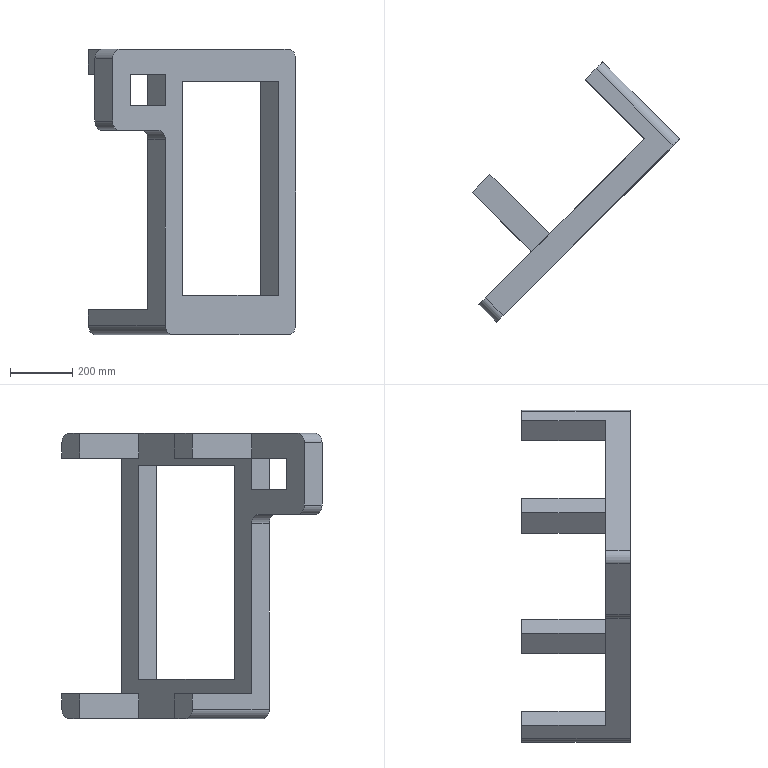Part | SolidWorks | 1 solid | 36 faces | box 666.188 x 835.894 x 917.42 mm | volume 30070373 mm3 | plane 30 | cylinder 6 | commonest cylinder face diameters 60 x6
STEP:
#1=CARTESIAN_POINT('',(-502.046,346.482,64.5));
#2=VERTEX_POINT('',#1);
#3=CARTESIAN_POINT('',(-502.046,346.482,-15.5));
#4=VERTEX_POINT('',#3);
#5=CARTESIAN_POINT('',(-502.046,346.482,64.5));
#6=DIRECTION('',(0.,0.,-1.));
#7=VECTOR('',#6,1000.);
#8=LINE('',#5,#7);
#9=EDGE_CURVE('',#2,#4,#8,.T.);
#10=ORIENTED_EDGE('',*,*,#9,.T.);
#11=CARTESIAN_POINT('',(-558.614,289.914,-15.5));
#12=VERTEX_POINT('',#11);
#13=CARTESIAN_POINT('',(-502.046,346.482,-15.5));
#14=DIRECTION('',(-0.7071,-0.7071,0.));
#15=VECTOR('',#14,1000.);
#16=LINE('',#13,#15);
#17=EDGE_CURVE('',#4,#12,#16,.T.);
#18=ORIENTED_EDGE('',*,*,#17,.T.);
#19=CARTESIAN_POINT('',(-558.614,289.914,64.5));
#20=VERTEX_POINT('',#19);
#21=CARTESIAN_POINT('',(-558.614,289.914,-15.5));
#22=DIRECTION('',(0.,0.,1.));
#23=VECTOR('',#22,1000.);
#24=LINE('',#21,#23);
#25=EDGE_CURVE('',#12,#20,#24,.T.);
#26=ORIENTED_EDGE('',*,*,#25,.T.);
#27=CARTESIAN_POINT('',(-558.614,289.914,64.5));
#28=DIRECTION('',(0.7071,0.7071,0.));
#29=VECTOR('',#28,1000.);
#30=LINE('',#27,#29);
#31=EDGE_CURVE('',#20,#2,#30,.T.);
#32=ORIENTED_EDGE('',*,*,#31,.T.);
#33=EDGE_LOOP('',(#10,#18,#26,#32));
#34=FACE_OUTER_BOUND('',#33,.T.);
#35=CARTESIAN_POINT('',(-424.264,424.264,0.));
#36=DIRECTION('',(-0.7071,0.7071,0.));
#37=DIRECTION('',(-0.7071,-0.7071,0.));
#38=AXIS2_PLACEMENT_3D('',#35,#36,#37);
#39=PLANE('',#38);
#40=ADVANCED_FACE('',(#34),#39,.T.);
#41=CARTESIAN_POINT('',(-311.127,155.563,64.5));
#42=VERTEX_POINT('',#41);
#43=CARTESIAN_POINT('',(-311.127,155.563,64.5));
#44=DIRECTION('',(-0.7071,0.7071,0.));
#45=VECTOR('',#44,1000.);
#46=LINE('',#43,#45);
#47=EDGE_CURVE('',#42,#2,#46,.T.);
#48=ORIENTED_EDGE('',*,*,#47,.T.);
#49=ORIENTED_EDGE('',*,*,#31,.F.);
#50=CARTESIAN_POINT('',(-367.696,98.995,64.5));
#51=VERTEX_POINT('',#50);
#52=CARTESIAN_POINT('',(-367.696,98.995,64.5));
#53=DIRECTION('',(-0.7071,0.7071,0.));
#54=VECTOR('',#53,1000.);
#55=LINE('',#52,#54);
#56=EDGE_CURVE('',#51,#20,#55,.T.);
#57=ORIENTED_EDGE('',*,*,#56,.F.);
#58=CARTESIAN_POINT('',(-367.696,98.995,64.5));
#59=DIRECTION('',(0.7071,0.7071,0.));
#60=VECTOR('',#59,1000.);
#61=LINE('',#58,#60);
#62=EDGE_CURVE('',#51,#42,#61,.T.);
#63=ORIENTED_EDGE('',*,*,#62,.T.);
#64=EDGE_LOOP('',(#48,#49,#57,#63));
#65=FACE_OUTER_BOUND('',#64,.T.);
#66=CARTESIAN_POINT('',(-311.127,42.426,64.5));
#67=DIRECTION('',(0.,0.,1.));
#68=DIRECTION('',(0.7071,0.7071,0.));
#69=AXIS2_PLACEMENT_3D('',#66,#67,#68);
#70=PLANE('',#69);
#71=ADVANCED_FACE('',(#65),#70,.T.);
#72=CARTESIAN_POINT('',(-311.127,155.563,-15.5));
#73=VERTEX_POINT('',#72);
#74=CARTESIAN_POINT('',(-311.127,155.563,-15.5));
#75=DIRECTION('',(-0.7071,0.7071,0.));
#76=VECTOR('',#75,1000.);
#77=LINE('',#74,#76);
#78=EDGE_CURVE('',#73,#4,#77,.T.);
#79=ORIENTED_EDGE('',*,*,#78,.T.);
#80=ORIENTED_EDGE('',*,*,#9,.F.);
#81=ORIENTED_EDGE('',*,*,#47,.F.);
#82=CARTESIAN_POINT('',(-311.127,155.563,64.5));
#83=DIRECTION('',(0.,0.,-1.));
#84=VECTOR('',#83,1000.);
#85=LINE('',#82,#84);
#86=EDGE_CURVE('',#42,#73,#85,.T.);
#87=ORIENTED_EDGE('',*,*,#86,.T.);
#88=EDGE_LOOP('',(#79,#80,#81,#87));
#89=FACE_OUTER_BOUND('',#88,.T.);
#90=CARTESIAN_POINT('',(-254.558,98.995,64.5));
#91=DIRECTION('',(0.7071,0.7071,0.));
#92=DIRECTION('',(0.,0.,-1.));
#93=AXIS2_PLACEMENT_3D('',#90,#91,#92);
#94=PLANE('',#93);
#95=ADVANCED_FACE('',(#89),#94,.T.);
#96=ORIENTED_EDGE('',*,*,#17,.F.);
#97=ORIENTED_EDGE('',*,*,#78,.F.);
#98=CARTESIAN_POINT('',(-367.696,98.995,-15.5));
#99=VERTEX_POINT('',#98);
#100=CARTESIAN_POINT('',(-311.127,155.563,-15.5));
#101=DIRECTION('',(-0.7071,-0.7071,0.));
#102=VECTOR('',#101,1000.);
#103=LINE('',#100,#102);
#104=EDGE_CURVE('',#73,#99,#103,.T.);
#105=ORIENTED_EDGE('',*,*,#104,.T.);
#106=CARTESIAN_POINT('',(-367.696,98.995,-15.5));
#107=DIRECTION('',(-0.7071,0.7071,0.));
#108=VECTOR('',#107,1000.);
#109=LINE('',#106,#108);
#110=EDGE_CURVE('',#99,#12,#109,.T.);
#111=ORIENTED_EDGE('',*,*,#110,.T.);
#112=EDGE_LOOP('',(#96,#97,#105,#111));
#113=FACE_OUTER_BOUND('',#112,.T.);
#114=CARTESIAN_POINT('',(-254.558,98.995,-15.5));
#115=DIRECTION('',(0.,0.,-1.));
#116=DIRECTION('',(-0.7071,-0.7071,0.));
#117=AXIS2_PLACEMENT_3D('',#114,#115,#116);
#118=PLANE('',#117);
#119=ADVANCED_FACE('',(#113),#118,.T.);
#120=ORIENTED_EDGE('',*,*,#56,.T.);
#121=ORIENTED_EDGE('',*,*,#25,.F.);
#122=ORIENTED_EDGE('',*,*,#110,.F.);
#123=CARTESIAN_POINT('',(-367.696,98.995,64.5));
#124=DIRECTION('',(0.,0.,-1.));
#125=VECTOR('',#124,1000.);
#126=LINE('',#123,#125);
#127=EDGE_CURVE('',#51,#99,#126,.T.);
#128=ORIENTED_EDGE('',*,*,#127,.F.);
#129=EDGE_LOOP('',(#120,#121,#122,#128));
#130=FACE_OUTER_BOUND('',#129,.T.);
#131=CARTESIAN_POINT('',(-311.127,42.426,-15.5));
#132=DIRECTION('',(-0.7071,-0.7071,0.));
#133=DIRECTION('',(0.,0.,1.));
#134=AXIS2_PLACEMENT_3D('',#131,#132,#133);
#135=PLANE('',#134);
#136=ADVANCED_FACE('',(#130),#135,.T.);
#137=CARTESIAN_POINT('',(-367.696,98.995,-115.5));
#138=VERTEX_POINT('',#137);
#139=CARTESIAN_POINT('',(-367.696,98.995,-15.5));
#140=DIRECTION('',(0.,0.,-1.));
#141=VECTOR('',#140,1000.);
#142=LINE('',#139,#141);
#143=EDGE_CURVE('',#99,#138,#142,.T.);
#144=ORIENTED_EDGE('',*,*,#143,.T.);
#145=CARTESIAN_POINT('',(-311.127,42.426,-115.5));
#146=VERTEX_POINT('',#145);
#147=CARTESIAN_POINT('',(-311.127,42.426,-115.5));
#148=DIRECTION('',(-0.7071,0.7071,0.));
#149=VECTOR('',#148,1000.);
#150=LINE('',#147,#149);
#151=EDGE_CURVE('',#146,#138,#150,.T.);
#152=ORIENTED_EDGE('',*,*,#151,.F.);
#153=CARTESIAN_POINT('',(-311.127,42.426,-15.5));
#154=VERTEX_POINT('',#153);
#155=CARTESIAN_POINT('',(-311.127,42.426,-15.5));
#156=DIRECTION('',(0.,0.,-1.));
#157=VECTOR('',#156,1000.);
#158=LINE('',#155,#157);
#159=EDGE_CURVE('',#154,#146,#158,.T.);
#160=ORIENTED_EDGE('',*,*,#159,.F.);
#161=CARTESIAN_POINT('',(-311.127,42.426,-15.5));
#162=DIRECTION('',(-0.7071,0.7071,0.));
#163=VECTOR('',#162,1000.);
#164=LINE('',#161,#163);
#165=EDGE_CURVE('',#154,#99,#164,.T.);
#166=ORIENTED_EDGE('',*,*,#165,.T.);
#167=EDGE_LOOP('',(#144,#152,#160,#166));
#168=FACE_OUTER_BOUND('',#167,.T.);
#169=CARTESIAN_POINT('',(-311.127,42.426,-15.5));
#170=DIRECTION('',(-0.7071,-0.7071,0.));
#171=DIRECTION('',(0.,0.,1.));
#172=AXIS2_PLACEMENT_3D('',#169,#170,#171);
#173=PLANE('',#172);
#174=ADVANCED_FACE('',(#168),#173,.T.);
#175=CARTESIAN_POINT('',(-424.264,-70.711,-115.5));
#176=VERTEX_POINT('',#175);
#177=CARTESIAN_POINT('',(-311.127,42.426,-115.5));
#178=DIRECTION('',(-0.7071,-0.7071,0.));
#179=VECTOR('',#178,1000.);
#180=LINE('',#177,#179);
#181=EDGE_CURVE('',#146,#176,#180,.T.);
#182=ORIENTED_EDGE('',*,*,#181,.F.);
#183=ORIENTED_EDGE('',*,*,#151,.T.);
#184=CARTESIAN_POINT('',(-480.833,-14.142,-115.5));
#185=VERTEX_POINT('',#184);
#186=CARTESIAN_POINT('',(-367.696,98.995,-115.5));
#187=DIRECTION('',(-0.7071,-0.7071,0.));
#188=VECTOR('',#187,1000.);
#189=LINE('',#186,#188);
#190=EDGE_CURVE('',#138,#185,#189,.T.);
#191=ORIENTED_EDGE('',*,*,#190,.T.);
#192=CARTESIAN_POINT('',(-424.264,-70.711,-115.5));
#193=DIRECTION('',(-0.7071,0.7071,0.));
#194=VECTOR('',#193,1000.);
#195=LINE('',#192,#194);
#196=EDGE_CURVE('',#176,#185,#195,.T.);
#197=ORIENTED_EDGE('',*,*,#196,.F.);
#198=EDGE_LOOP('',(#182,#183,#191,#197));
#199=FACE_OUTER_BOUND('',#198,.T.);
#200=CARTESIAN_POINT('',(-311.127,42.426,-115.5));
#201=DIRECTION('',(0.,0.,1.));
#202=DIRECTION('',(-0.7071,0.7071,0.));
#203=AXIS2_PLACEMENT_3D('',#200,#201,#202);
#204=PLANE('',#203);
#205=ADVANCED_FACE('',(#199),#204,.T.);
#206=CARTESIAN_POINT('',(-424.264,-70.711,-15.5));
#207=VERTEX_POINT('',#206);
#208=CARTESIAN_POINT('',(-424.264,-70.711,-15.5));
#209=DIRECTION('',(0.,0.,-1.));
#210=VECTOR('',#209,1000.);
#211=LINE('',#208,#210);
#212=EDGE_CURVE('',#207,#176,#211,.T.);
#213=ORIENTED_EDGE('',*,*,#212,.T.);
#214=ORIENTED_EDGE('',*,*,#196,.T.);
#215=CARTESIAN_POINT('',(-480.833,-14.142,-15.5));
#216=VERTEX_POINT('',#215);
#217=CARTESIAN_POINT('',(-480.833,-14.142,-15.5));
#218=DIRECTION('',(0.,0.,-1.));
#219=VECTOR('',#218,1000.);
#220=LINE('',#217,#219);
#221=EDGE_CURVE('',#216,#185,#220,.T.);
#222=ORIENTED_EDGE('',*,*,#221,.F.);
#223=CARTESIAN_POINT('',(-480.833,-14.142,-15.5));
#224=DIRECTION('',(0.7071,-0.7071,0.));
#225=VECTOR('',#224,1000.);
#226=LINE('',#223,#225);
#227=EDGE_CURVE('',#216,#207,#226,.T.);
#228=ORIENTED_EDGE('',*,*,#227,.T.);
#229=EDGE_LOOP('',(#213,#214,#222,#228));
#230=FACE_OUTER_BOUND('',#229,.T.);
#231=CARTESIAN_POINT('',(-424.264,-70.711,65.));
#232=DIRECTION('',(0.7071,0.7071,0.));
#233=DIRECTION('',(-0.7071,0.7071,0.));
#234=AXIS2_PLACEMENT_3D('',#231,#232,#233);
#235=PLANE('',#234);
#236=ADVANCED_FACE('',(#230),#235,.T.);
#237=CARTESIAN_POINT('',(-367.696,98.995,-15.5));
#238=DIRECTION('',(-0.7071,-0.7071,0.));
#239=VECTOR('',#238,1000.);
#240=LINE('',#237,#239);
#241=EDGE_CURVE('',#99,#216,#240,.T.);
#242=ORIENTED_EDGE('',*,*,#241,.F.);
#243=ORIENTED_EDGE('',*,*,#165,.F.);
#244=CARTESIAN_POINT('',(-311.127,42.426,-15.5));
#245=DIRECTION('',(-0.7071,-0.7071,0.));
#246=VECTOR('',#245,1000.);
#247=LINE('',#244,#246);
#248=EDGE_CURVE('',#154,#207,#247,.T.);
#249=ORIENTED_EDGE('',*,*,#248,.T.);
#250=ORIENTED_EDGE('',*,*,#227,.F.);
#251=EDGE_LOOP('',(#242,#243,#249,#250));
#252=FACE_OUTER_BOUND('',#251,.T.);
#253=CARTESIAN_POINT('',(-367.696,98.995,-15.5));
#254=DIRECTION('',(0.,0.,-1.));
#255=DIRECTION('',(0.7071,-0.7071,0.));
#256=AXIS2_PLACEMENT_3D('',#253,#254,#255);
#257=PLANE('',#256);
#258=ADVANCED_FACE('',(#252),#257,.T.);
#259=CARTESIAN_POINT('',(51.005,404.558,-726.128));
#260=VERTEX_POINT('',#259);
#261=CARTESIAN_POINT('',(-254.558,98.995,-726.128));
#262=VERTEX_POINT('',#261);
#263=CARTESIAN_POINT('',(51.005,404.558,-726.128));
#264=DIRECTION('',(-0.7071,-0.7071,0.));
#265=VECTOR('',#264,1000.);
#266=LINE('',#263,#265);
#267=EDGE_CURVE('',#260,#262,#266,.T.);
#268=ORIENTED_EDGE('',*,*,#267,.F.);
#269=CARTESIAN_POINT('',(-5.563,461.127,-726.128));
#270=VERTEX_POINT('',#269);
#271=CARTESIAN_POINT('',(51.005,404.558,-726.128));
#272=DIRECTION('',(-0.7071,0.7071,0.));
#273=VECTOR('',#272,1000.);
#274=LINE('',#271,#273);
#275=EDGE_CURVE('',#260,#270,#274,.T.);
#276=ORIENTED_EDGE('',*,*,#275,.T.);
#277=CARTESIAN_POINT('',(-311.127,155.563,-726.128));
#278=VERTEX_POINT('',#277);
#279=CARTESIAN_POINT('',(-5.563,461.127,-726.128));
#280=DIRECTION('',(-0.7071,-0.7071,0.));
#281=VECTOR('',#280,1000.);
#282=LINE('',#279,#281);
#283=EDGE_CURVE('',#270,#278,#282,.T.);
#284=ORIENTED_EDGE('',*,*,#283,.T.);
#285=CARTESIAN_POINT('',(-254.558,98.995,-726.128));
#286=DIRECTION('',(-0.7071,0.7071,0.));
#287=VECTOR('',#286,1000.);
#288=LINE('',#285,#287);
#289=EDGE_CURVE('',#262,#278,#288,.T.);
#290=ORIENTED_EDGE('',*,*,#289,.F.);
#291=EDGE_LOOP('',(#268,#276,#284,#290));
#292=FACE_OUTER_BOUND('',#291,.T.);
#293=CARTESIAN_POINT('',(51.005,517.696,-726.128));
#294=DIRECTION('',(0.,0.,1.));
#295=DIRECTION('',(0.7071,-0.7071,0.));
#296=AXIS2_PLACEMENT_3D('',#293,#294,#295);
#297=PLANE('',#296);
#298=ADVANCED_FACE('',(#292),#297,.T.);
#299=CARTESIAN_POINT('',(-5.563,461.127,-37.575));
#300=VERTEX_POINT('',#299);
#301=CARTESIAN_POINT('',(-5.563,461.127,-37.575));
#302=DIRECTION('',(0.,0.,-1.));
#303=VECTOR('',#302,1000.);
#304=LINE('',#301,#303);
#305=EDGE_CURVE('',#300,#270,#304,.T.);
#306=ORIENTED_EDGE('',*,*,#305,.T.);
#307=ORIENTED_EDGE('',*,*,#275,.F.);
#308=CARTESIAN_POINT('',(51.005,404.558,-37.575));
#309=VERTEX_POINT('',#308);
#310=CARTESIAN_POINT('',(51.005,404.558,-37.575));
#311=DIRECTION('',(0.,0.,-1.));
#312=VECTOR('',#311,1000.);
#313=LINE('',#310,#312);
#314=EDGE_CURVE('',#309,#260,#313,.T.);
#315=ORIENTED_EDGE('',*,*,#314,.F.);
#316=CARTESIAN_POINT('',(51.005,404.558,-37.575));
#317=DIRECTION('',(-0.7071,0.7071,0.));
#318=VECTOR('',#317,1000.);
#319=LINE('',#316,#318);
#320=EDGE_CURVE('',#309,#300,#319,.T.);
#321=ORIENTED_EDGE('',*,*,#320,.T.);
#322=EDGE_LOOP('',(#306,#307,#315,#321));
#323=FACE_OUTER_BOUND('',#322,.T.);
#324=CARTESIAN_POINT('',(51.005,404.558,-852.42));
#325=DIRECTION('',(-0.7071,-0.7071,0.));
#326=DIRECTION('',(0.,0.,1.));
#327=AXIS2_PLACEMENT_3D('',#324,#325,#326);
#328=PLANE('',#327);
#329=ADVANCED_FACE('',(#323),#328,.T.);
#330=CARTESIAN_POINT('',(-311.127,155.563,-37.575));
#331=VERTEX_POINT('',#330);
#332=CARTESIAN_POINT('',(-5.563,461.127,-37.575));
#333=DIRECTION('',(-0.7071,-0.7071,0.));
#334=VECTOR('',#333,1000.);
#335=LINE('',#332,#334);
#336=EDGE_CURVE('',#300,#331,#335,.T.);
#337=ORIENTED_EDGE('',*,*,#336,.F.);
#338=ORIENTED_EDGE('',*,*,#320,.F.);
#339=CARTESIAN_POINT('',(-254.558,98.995,-37.575));
#340=VERTEX_POINT('',#339);
#341=CARTESIAN_POINT('',(51.005,404.558,-37.575));
#342=DIRECTION('',(-0.7071,-0.7071,0.));
#343=VECTOR('',#342,1000.);
#344=LINE('',#341,#343);
#345=EDGE_CURVE('',#309,#340,#344,.T.);
#346=ORIENTED_EDGE('',*,*,#345,.T.);
#347=CARTESIAN_POINT('',(-254.558,98.995,-37.575));
#348=DIRECTION('',(-0.7071,0.7071,0.));
#349=VECTOR('',#348,1000.);
#350=LINE('',#347,#349);
#351=EDGE_CURVE('',#340,#331,#350,.T.);
#352=ORIENTED_EDGE('',*,*,#351,.T.);
#353=EDGE_LOOP('',(#337,#338,#346,#352));
#354=FACE_OUTER_BOUND('',#353,.T.);
#355=CARTESIAN_POINT('',(107.574,461.127,-37.575));
#356=DIRECTION('',(0.,0.,-1.));
#357=DIRECTION('',(-0.7071,0.7071,0.));
#358=AXIS2_PLACEMENT_3D('',#355,#356,#357);
#359=PLANE('',#358);
#360=ADVANCED_FACE('',(#354),#359,.T.);
#361=CARTESIAN_POINT('',(-254.558,98.995,-37.575));
#362=DIRECTION('',(0.,0.,-1.));
#363=VECTOR('',#362,1000.);
#364=LINE('',#361,#363);
#365=EDGE_CURVE('',#340,#262,#364,.T.);
#366=ORIENTED_EDGE('',*,*,#365,.T.);
#367=ORIENTED_EDGE('',*,*,#289,.T.);
#368=CARTESIAN_POINT('',(-311.127,155.563,-37.575));
#369=DIRECTION('',(0.,0.,-1.));
#370=VECTOR('',#369,1000.);
#371=LINE('',#368,#370);
#372=EDGE_CURVE('',#331,#278,#371,.T.);
#373=ORIENTED_EDGE('',*,*,#372,.F.);
#374=ORIENTED_EDGE('',*,*,#351,.F.);
#375=EDGE_LOOP('',(#366,#367,#373,#374));
#376=FACE_OUTER_BOUND('',#375,.T.);
#377=CARTESIAN_POINT('',(-254.558,98.995,64.5));
#378=DIRECTION('',(0.7071,0.7071,0.));
#379=DIRECTION('',(0.,0.,-1.));
#380=AXIS2_PLACEMENT_3D('',#377,#378,#379);
#381=PLANE('',#380);
#382=ADVANCED_FACE('',(#376),#381,.T.);
#383=CARTESIAN_POINT('',(-5.563,461.127,-15.));
#384=VERTEX_POINT('',#383);
#385=CARTESIAN_POINT('',(-196.482,652.046,-15.));
#386=VERTEX_POINT('',#385);
#387=CARTESIAN_POINT('',(-5.563,461.127,-15.));
#388=DIRECTION('',(-0.7071,0.7071,0.));
#389=VECTOR('',#388,1000.);
#390=LINE('',#387,#389);
#391=EDGE_CURVE('',#384,#386,#390,.T.);
#392=ORIENTED_EDGE('',*,*,#391,.T.);
#393=CARTESIAN_POINT('',(-139.914,708.614,-15.));
#394=VERTEX_POINT('',#393);
#395=CARTESIAN_POINT('',(-139.914,708.614,-15.));
#396=DIRECTION('',(-0.7071,-0.7071,0.));
#397=VECTOR('',#396,1000.);
#398=LINE('',#395,#397);
#399=EDGE_CURVE('',#394,#386,#398,.T.);
#400=ORIENTED_EDGE('',*,*,#399,.F.);
#401=CARTESIAN_POINT('',(51.005,517.696,-15.));
#402=VERTEX_POINT('',#401);
#403=CARTESIAN_POINT('',(51.005,517.696,-15.));
#404=DIRECTION('',(-0.7071,0.7071,0.));
#405=VECTOR('',#404,1000.);
#406=LINE('',#403,#405);
#407=EDGE_CURVE('',#402,#394,#406,.T.);
#408=ORIENTED_EDGE('',*,*,#407,.F.);
#409=CARTESIAN_POINT('',(51.005,517.696,-15.));
#410=DIRECTION('',(-0.7071,-0.7071,0.));
#411=VECTOR('',#410,1000.);
#412=LINE('',#409,#411);
#413=EDGE_CURVE('',#402,#384,#412,.T.);
#414=ORIENTED_EDGE('',*,*,#413,.T.);
#415=EDGE_LOOP('',(#392,#400,#408,#414));
#416=FACE_OUTER_BOUND('',#415,.T.);
#417=CARTESIAN_POINT('',(107.574,461.127,-15.));
#418=DIRECTION('',(0.,0.,-1.));
#419=DIRECTION('',(-0.7071,-0.7071,0.));
#420=AXIS2_PLACEMENT_3D('',#417,#418,#419);
#421=PLANE('',#420);
#422=ADVANCED_FACE('',(#416),#421,.T.);
#423=CARTESIAN_POINT('',(-502.046,346.482,-852.42));
#424=VERTEX_POINT('',#423);
#425=CARTESIAN_POINT('',(-537.401,311.127,-852.42));
#426=VERTEX_POINT('',#425);
#427=CARTESIAN_POINT('',(-502.046,346.482,-852.42));
#428=DIRECTION('',(-0.7071,-0.7071,0.));
#429=VECTOR('',#428,1000.);
#430=LINE('',#427,#429);
#431=EDGE_CURVE('',#424,#426,#430,.T.);
#432=ORIENTED_EDGE('',*,*,#431,.T.);
#433=CARTESIAN_POINT('',(-558.614,289.914,-822.42));
#434=VERTEX_POINT('',#433);
#435=CARTESIAN_POINT('',(-537.401,311.127,-822.42));
#436=DIRECTION('',(-0.7071,0.7071,0.));
#437=DIRECTION('',(-0.7071,-0.7071,0.));
#438=AXIS2_PLACEMENT_3D('',#435,#436,#437);
#439=CIRCLE('',#438,30.);
#440=EDGE_CURVE('',#426,#434,#439,.T.);
#441=ORIENTED_EDGE('',*,*,#440,.T.);
#442=CARTESIAN_POINT('',(-558.614,289.914,-772.42));
#443=VERTEX_POINT('',#442);
#444=CARTESIAN_POINT('',(-558.614,289.914,-852.42));
#445=DIRECTION('',(0.,0.,1.));
#446=VECTOR('',#445,1000.);
#447=LINE('',#444,#446);
#448=EDGE_CURVE('',#434,#443,#447,.T.);
#449=ORIENTED_EDGE('',*,*,#448,.T.);
#450=CARTESIAN_POINT('',(-502.046,346.482,-772.42));
#451=VERTEX_POINT('',#450);
#452=CARTESIAN_POINT('',(-558.614,289.914,-772.42));
#453=DIRECTION('',(0.7071,0.7071,0.));
#454=VECTOR('',#453,1000.);
#455=LINE('',#452,#454);
#456=EDGE_CURVE('',#443,#451,#455,.T.);
#457=ORIENTED_EDGE('',*,*,#456,.T.);
#458=CARTESIAN_POINT('',(-502.046,346.482,-772.42));
#459=DIRECTION('',(0.,0.,-1.));
#460=VECTOR('',#459,1000.);
#461=LINE('',#458,#460);
#462=EDGE_CURVE('',#451,#424,#461,.T.);
#463=ORIENTED_EDGE('',*,*,#462,.T.);
#464=EDGE_LOOP('',(#432,#441,#449,#457,#463));
#465=FACE_OUTER_BOUND('',#464,.T.);
#466=CARTESIAN_POINT('',(-424.264,424.264,0.));
#467=DIRECTION('',(-0.7071,0.7071,0.));
#468=DIRECTION('',(-0.7071,-0.7071,0.));
#469=AXIS2_PLACEMENT_3D('',#466,#467,#468);
#470=PLANE('',#469);
#471=ADVANCED_FACE('',(#465),#470,.T.);
#472=CARTESIAN_POINT('',(-332.34,21.213,-195.5));
#473=VERTEX_POINT('',#472);
#474=CARTESIAN_POINT('',(-459.619,-106.066,-195.5));
#475=VERTEX_POINT('',#474);
#476=CARTESIAN_POINT('',(-311.127,42.426,-195.5));
#477=DIRECTION('',(-0.7071,-0.7071,0.));
#478=VECTOR('',#477,1000.);
#479=LINE('',#476,#478);
#480=EDGE_CURVE('',#473,#475,#479,.T.);
#481=ORIENTED_EDGE('',*,*,#480,.T.);
#482=CARTESIAN_POINT('',(-516.188,-49.497,-195.5));
#483=VERTEX_POINT('',#482);
#484=CARTESIAN_POINT('',(-516.188,-49.497,-195.5));
#485=DIRECTION('',(-0.7071,0.7071,0.));
#486=VECTOR('',#485,1000.);
#487=LINE('',#484,#486);
#488=EDGE_CURVE('',#475,#483,#487,.T.);
#489=ORIENTED_EDGE('',*,*,#488,.T.);
#490=CARTESIAN_POINT('',(-388.909,77.782,-195.5));
#491=VERTEX_POINT('',#490);
#492=CARTESIAN_POINT('',(-367.696,98.995,-195.5));
#493=DIRECTION('',(-0.7071,-0.7071,0.));
#494=VECTOR('',#493,1000.);
#495=LINE('',#492,#494);
#496=EDGE_CURVE('',#491,#483,#495,.T.);
#497=ORIENTED_EDGE('',*,*,#496,.F.);
#498=CARTESIAN_POINT('',(-332.34,21.213,-195.5));
#499=DIRECTION('',(0.7071,-0.7071,0.));
#500=VECTOR('',#499,1000.);
#501=LINE('',#498,#500);
#502=EDGE_CURVE('',#491,#473,#501,.T.);
#503=ORIENTED_EDGE('',*,*,#502,.T.);
#504=EDGE_LOOP('',(#481,#489,#497,#503));
#505=FACE_OUTER_BOUND('',#504,.T.);
#506=CARTESIAN_POINT('',(-367.696,98.995,-195.5));
#507=DIRECTION('',(0.,0.,-1.));
#508=DIRECTION('',(0.7071,-0.7071,0.));
#509=AXIS2_PLACEMENT_3D('',#506,#507,#508);
#510=PLANE('',#509);
#511=ADVANCED_FACE('',(#505),#510,.T.);
#512=ORIENTED_EDGE('',*,*,#448,.F.);
#513=CARTESIAN_POINT('',(-311.127,42.426,-822.42));
#514=VERTEX_POINT('',#513);
#515=CARTESIAN_POINT('',(-311.127,42.426,-822.42));
#516=DIRECTION('',(0.7071,-0.7071,0.));
#517=VECTOR('',#516,1000.);
#518=LINE('',#515,#517);
#519=EDGE_CURVE('',#434,#514,#518,.T.);
#520=ORIENTED_EDGE('',*,*,#519,.T.);
#521=CARTESIAN_POINT('',(-311.127,42.426,-225.5));
#522=VERTEX_POINT('',#521);
#523=CARTESIAN_POINT('',(-311.127,42.426,-195.5));
#524=DIRECTION('',(0.,0.,-1.));
#525=VECTOR('',#524,1000.);
#526=LINE('',#523,#525);
#527=EDGE_CURVE('',#522,#514,#526,.T.);
#528=ORIENTED_EDGE('',*,*,#527,.F.);
#529=CARTESIAN_POINT('',(-367.696,98.995,-225.5));
#530=VERTEX_POINT('',#529);
#531=CARTESIAN_POINT('',(-367.696,98.995,-225.5));
#532=DIRECTION('',(-0.7071,0.7071,0.));
#533=VECTOR('',#532,1000.);
#534=LINE('',#531,#533);
#535=EDGE_CURVE('',#522,#530,#534,.T.);
#536=ORIENTED_EDGE('',*,*,#535,.T.);
#537=CARTESIAN_POINT('',(-367.696,98.995,-772.42));
#538=VERTEX_POINT('',#537);
#539=CARTESIAN_POINT('',(-367.696,98.995,-195.5));
#540=DIRECTION('',(0.,0.,-1.));
#541=VECTOR('',#540,1000.);
#542=LINE('',#539,#541);
#543=EDGE_CURVE('',#530,#538,#542,.T.);
#544=ORIENTED_EDGE('',*,*,#543,.T.);
#545=CARTESIAN_POINT('',(-367.696,98.995,-772.42));
#546=DIRECTION('',(-0.7071,0.7071,0.));
#547=VECTOR('',#546,1000.);
#548=LINE('',#545,#547);
#549=EDGE_CURVE('',#538,#443,#548,.T.);
#550=ORIENTED_EDGE('',*,*,#549,.T.);
#551=EDGE_LOOP('',(#512,#520,#528,#536,#544,#550));
#552=FACE_OUTER_BOUND('',#551,.T.);
#553=CARTESIAN_POINT('',(-311.127,42.426,-15.5));
#554=DIRECTION('',(-0.7071,-0.7071,0.));
#555=DIRECTION('',(0.,0.,1.));
#556=AXIS2_PLACEMENT_3D('',#553,#554,#555);
#557=PLANE('',#556);
#558=ADVANCED_FACE('',(#552),#557,.T.);
#559=CARTESIAN_POINT('',(-311.127,155.563,-772.42));
#560=VERTEX_POINT('',#559);
#561=CARTESIAN_POINT('',(-311.127,155.563,-772.42));
#562=DIRECTION('',(-0.7071,0.7071,0.));
#563=VECTOR('',#562,1000.);
#564=LINE('',#561,#563);
#565=EDGE_CURVE('',#560,#451,#564,.T.);
#566=ORIENTED_EDGE('',*,*,#565,.T.);
#567=ORIENTED_EDGE('',*,*,#456,.F.);
#568=ORIENTED_EDGE('',*,*,#549,.F.);
#569=CARTESIAN_POINT('',(-367.696,98.995,-772.42));
#570=DIRECTION('',(0.7071,0.7071,0.));
#571=VECTOR('',#570,1000.);
#572=LINE('',#569,#571);
#573=EDGE_CURVE('',#538,#560,#572,.T.);
#574=ORIENTED_EDGE('',*,*,#573,.T.);
#575=EDGE_LOOP('',(#566,#567,#568,#574));
#576=FACE_OUTER_BOUND('',#575,.T.);
#577=CARTESIAN_POINT('',(-311.127,42.426,-772.42));
#578=DIRECTION('',(0.,0.,1.));
#579=DIRECTION('',(0.7071,0.7071,0.));
#580=AXIS2_PLACEMENT_3D('',#577,#578,#579);
#581=PLANE('',#580);
#582=ADVANCED_FACE('',(#576),#581,.T.);
#583=CARTESIAN_POINT('',(-311.127,155.563,-852.42));
#584=VERTEX_POINT('',#583);
#585=CARTESIAN_POINT('',(-311.127,155.563,-852.42));
#586=DIRECTION('',(-0.7071,0.7071,0.));
#587=VECTOR('',#586,1000.);
#588=LINE('',#585,#587);
#589=EDGE_CURVE('',#584,#424,#588,.T.);
#590=ORIENTED_EDGE('',*,*,#589,.T.);
#591=ORIENTED_EDGE('',*,*,#462,.F.);
#592=ORIENTED_EDGE('',*,*,#565,.F.);
#593=CARTESIAN_POINT('',(-311.127,155.563,-852.42));
#594=DIRECTION('',(0.,0.,1.));
#595=VECTOR('',#594,1000.);
#596=LINE('',#593,#595);
#597=EDGE_CURVE('',#584,#560,#596,.T.);
#598=ORIENTED_EDGE('',*,*,#597,.F.);
#599=EDGE_LOOP('',(#590,#591,#592,#598));
#600=FACE_OUTER_BOUND('',#599,.T.);
#601=CARTESIAN_POINT('',(-254.558,98.995,64.5));
#602=DIRECTION('',(0.7071,0.7071,0.));
#603=DIRECTION('',(0.,0.,-1.));
#604=AXIS2_PLACEMENT_3D('',#601,#602,#603);
#605=PLANE('',#604);
#606=ADVANCED_FACE('',(#600),#605,.T.);
#607=CARTESIAN_POINT('',(-139.914,708.614,-772.42));
#608=VERTEX_POINT('',#607);
#609=CARTESIAN_POINT('',(-139.914,708.614,-822.42));
#610=VERTEX_POINT('',#609);
#611=CARTESIAN_POINT('',(-139.914,708.614,-772.42));
#612=DIRECTION('',(0.,0.,-1.));
#613=VECTOR('',#612,1000.);
#614=LINE('',#611,#613);
#615=EDGE_CURVE('',#608,#610,#614,.T.);
#616=ORIENTED_EDGE('',*,*,#615,.T.);
#617=CARTESIAN_POINT('',(-161.127,687.401,-852.42));
#618=VERTEX_POINT('',#617);
#619=CARTESIAN_POINT('',(-161.127,687.401,-822.42));
#620=DIRECTION('',(-0.7071,0.7071,0.));
#621=DIRECTION('',(-0.7071,-0.7071,0.));
#622=AXIS2_PLACEMENT_3D('',#619,#620,#621);
#623=CIRCLE('',#622,30.);
#624=EDGE_CURVE('',#610,#618,#623,.T.);
#625=ORIENTED_EDGE('',*,*,#624,.T.);
#626=CARTESIAN_POINT('',(-196.482,652.046,-852.42));
#627=VERTEX_POINT('',#626);
#628=CARTESIAN_POINT('',(-139.914,708.614,-852.42));
#629=DIRECTION('',(-0.7071,-0.7071,0.));
#630=VECTOR('',#629,1000.);
#631=LINE('',#628,#630);
#632=EDGE_CURVE('',#618,#627,#631,.T.);
#633=ORIENTED_EDGE('',*,*,#632,.T.);
#634=CARTESIAN_POINT('',(-196.482,652.046,-772.42));
#635=VERTEX_POINT('',#634);
#636=CARTESIAN_POINT('',(-196.482,652.046,-852.42));
#637=DIRECTION('',(0.,0.,1.));
#638=VECTOR('',#637,1000.);
#639=LINE('',#636,#638);
#640=EDGE_CURVE('',#627,#635,#639,.T.);
#641=ORIENTED_EDGE('',*,*,#640,.T.);
#642=CARTESIAN_POINT('',(-196.482,652.046,-772.42));
#643=DIRECTION('',(0.7071,0.7071,0.));
#644=VECTOR('',#643,1000.);
#645=LINE('',#642,#644);
#646=EDGE_CURVE('',#635,#608,#645,.T.);
#647=ORIENTED_EDGE('',*,*,#646,.T.);
#648=EDGE_LOOP('',(#616,#625,#633,#641,#647));
#649=FACE_OUTER_BOUND('',#648,.T.);
#650=CARTESIAN_POINT('',(-424.264,424.264,0.));
#651=DIRECTION('',(-0.7071,0.7071,0.));
#652=DIRECTION('',(-0.7071,-0.7071,0.));
#653=AXIS2_PLACEMENT_3D('',#650,#651,#652);
#654=PLANE('',#653);
#655=ADVANCED_FACE('',(#649),#654,.T.);
#656=CARTESIAN_POINT('',(-289.914,63.64,-852.42));
#657=VERTEX_POINT('',#656);
#658=CARTESIAN_POINT('',(86.36,439.914,-852.42));
#659=VERTEX_POINT('',#658);
#660=CARTESIAN_POINT('',(-311.127,42.426,-852.42));
#661=DIRECTION('',(0.7071,0.7071,0.));
#662=VECTOR('',#661,1000.);
#663=LINE('',#660,#662);
#664=EDGE_CURVE('',#657,#659,#663,.T.);
#665=ORIENTED_EDGE('',*,*,#664,.F.);
#666=CARTESIAN_POINT('',(-289.914,63.64,-852.42));
#667=DIRECTION('',(-0.7071,0.7071,0.));
#668=VECTOR('',#667,1000.);
#669=LINE('',#666,#668);
#670=EDGE_CURVE('',#657,#426,#669,.T.);
#671=ORIENTED_EDGE('',*,*,#670,.T.);
#672=ORIENTED_EDGE('',*,*,#431,.F.);
#673=ORIENTED_EDGE('',*,*,#589,.F.);
#674=CARTESIAN_POINT('',(-5.563,461.127,-852.42));
#675=VERTEX_POINT('',#674);
#676=CARTESIAN_POINT('',(-5.563,461.127,-852.42));
#677=DIRECTION('',(-0.7071,-0.7071,0.));
#678=VECTOR('',#677,1000.);
#679=LINE('',#676,#678);
#680=EDGE_CURVE('',#675,#584,#679,.T.);
#681=ORIENTED_EDGE('',*,*,#680,.F.);
#682=CARTESIAN_POINT('',(-5.563,461.127,-852.42));
#683=DIRECTION('',(-0.7071,0.7071,0.));
#684=VECTOR('',#683,1000.);
#685=LINE('',#682,#684);
#686=EDGE_CURVE('',#675,#627,#685,.T.);
#687=ORIENTED_EDGE('',*,*,#686,.T.);
#688=ORIENTED_EDGE('',*,*,#632,.F.);
#689=CARTESIAN_POINT('',(86.36,439.914,-852.42));
#690=DIRECTION('',(0.7071,-0.7071,0.));
#691=VECTOR('',#690,1000.);
#692=LINE('',#689,#691);
#693=EDGE_CURVE('',#618,#659,#692,.T.);
#694=ORIENTED_EDGE('',*,*,#693,.T.);
#695=EDGE_LOOP('',(#665,#671,#672,#673,#681,#687,#688,#694));
#696=FACE_OUTER_BOUND('',#695,.T.);
#697=CARTESIAN_POINT('',(-254.558,98.995,-852.42));
#698=DIRECTION('',(0.,0.,-1.));
#699=DIRECTION('',(-0.7071,-0.7071,0.));
#700=AXIS2_PLACEMENT_3D('',#697,#698,#699);
#701=PLANE('',#700);
#702=ADVANCED_FACE('',(#696),#701,.T.);
#703=CARTESIAN_POINT('',(-5.563,461.127,-772.42));
#704=VERTEX_POINT('',#703);
#705=CARTESIAN_POINT('',(-5.563,461.127,-772.42));
#706=DIRECTION('',(-0.7071,0.7071,0.));
#707=VECTOR('',#706,1000.);
#708=LINE('',#705,#707);
#709=EDGE_CURVE('',#704,#635,#708,.T.);
#710=ORIENTED_EDGE('',*,*,#709,.T.);
#711=ORIENTED_EDGE('',*,*,#640,.F.);
#712=ORIENTED_EDGE('',*,*,#686,.F.);
#713=CARTESIAN_POINT('',(-5.563,461.127,-852.42));
#714=DIRECTION('',(0.,0.,1.));
#715=VECTOR('',#714,1000.);
#716=LINE('',#713,#715);
#717=EDGE_CURVE('',#675,#704,#716,.T.);
#718=ORIENTED_EDGE('',*,*,#717,.T.);
#719=EDGE_LOOP('',(#710,#711,#712,#718));
#720=FACE_OUTER_BOUND('',#719,.T.);
#721=CARTESIAN_POINT('',(51.005,404.558,-852.42));
#722=DIRECTION('',(-0.7071,-0.7071,0.));
#723=DIRECTION('',(0.,0.,1.));
#724=AXIS2_PLACEMENT_3D('',#721,#722,#723);
#725=PLANE('',#724);
#726=ADVANCED_FACE('',(#720),#725,.T.);
#727=CARTESIAN_POINT('',(51.005,517.696,-772.42));
#728=VERTEX_POINT('',#727);
#729=CARTESIAN_POINT('',(51.005,517.696,-772.42));
#730=DIRECTION('',(-0.7071,0.7071,0.));
#731=VECTOR('',#730,1000.);
#732=LINE('',#729,#731);
#733=EDGE_CURVE('',#728,#608,#732,.T.);
#734=ORIENTED_EDGE('',*,*,#733,.T.);
#735=ORIENTED_EDGE('',*,*,#646,.F.);
#736=ORIENTED_EDGE('',*,*,#709,.F.);
#737=CARTESIAN_POINT('',(-5.563,461.127,-772.42));
#738=DIRECTION('',(0.7071,0.7071,0.));
#739=VECTOR('',#738,1000.);
#740=LINE('',#737,#739);
#741=EDGE_CURVE('',#704,#728,#740,.T.);
#742=ORIENTED_EDGE('',*,*,#741,.T.);
#743=EDGE_LOOP('',(#734,#735,#736,#742));
#744=FACE_OUTER_BOUND('',#743,.T.);
#745=CARTESIAN_POINT('',(51.005,404.558,-772.42));
#746=DIRECTION('',(0.,0.,1.));
#747=DIRECTION('',(0.7071,0.7071,0.));
#748=AXIS2_PLACEMENT_3D('',#745,#746,#747);
#749=PLANE('',#748);
#750=ADVANCED_FACE('',(#744),#749,.T.);
#751=CARTESIAN_POINT('',(-139.914,708.614,35.));
#752=VERTEX_POINT('',#751);
#753=CARTESIAN_POINT('',(-139.914,708.614,65.));
#754=DIRECTION('',(0.,0.,-1.));
#755=VECTOR('',#754,1000.);
#756=LINE('',#753,#755);
#757=EDGE_CURVE('',#752,#394,#756,.T.);
#758=ORIENTED_EDGE('',*,*,#757,.F.);
#759=CARTESIAN_POINT('',(107.574,461.127,35.));
#760=VERTEX_POINT('',#759);
#761=CARTESIAN_POINT('',(107.574,461.127,35.));
#762=DIRECTION('',(0.7071,-0.7071,0.));
#763=VECTOR('',#762,1000.);
#764=LINE('',#761,#763);
#765=EDGE_CURVE('',#752,#760,#764,.T.);
#766=ORIENTED_EDGE('',*,*,#765,.T.);
#767=CARTESIAN_POINT('',(107.574,461.127,-822.42));
#768=VERTEX_POINT('',#767);
#769=CARTESIAN_POINT('',(107.574,461.127,65.));
#770=DIRECTION('',(0.,0.,-1.));
#771=VECTOR('',#770,1000.);
#772=LINE('',#769,#771);
#773=EDGE_CURVE('',#760,#768,#772,.T.);
#774=ORIENTED_EDGE('',*,*,#773,.T.);
#775=CARTESIAN_POINT('',(107.574,461.127,-822.42));
#776=DIRECTION('',(-0.7071,0.7071,0.));
#777=VECTOR('',#776,1000.);
#778=LINE('',#775,#777);
#779=EDGE_CURVE('',#768,#610,#778,.T.);
#780=ORIENTED_EDGE('',*,*,#779,.T.);
#781=ORIENTED_EDGE('',*,*,#615,.F.);
#782=ORIENTED_EDGE('',*,*,#733,.F.);
#783=CARTESIAN_POINT('',(51.005,517.696,-772.42));
#784=DIRECTION('',(0.,0.,1.));
#785=VECTOR('',#784,1000.);
#786=LINE('',#783,#785);
#787=EDGE_CURVE('',#728,#402,#786,.T.);
#788=ORIENTED_EDGE('',*,*,#787,.T.);
#789=ORIENTED_EDGE('',*,*,#407,.T.);
#790=EDGE_LOOP('',(#758,#766,#774,#780,#781,#782,#788,#789));
#791=FACE_OUTER_BOUND('',#790,.T.);
#792=CARTESIAN_POINT('',(107.574,461.127,65.));
#793=DIRECTION('',(0.7071,0.7071,0.));
#794=DIRECTION('',(0.,0.,-1.));
#795=AXIS2_PLACEMENT_3D('',#792,#793,#794);
#796=PLANE('',#795);
#797=ADVANCED_FACE('',(#791),#796,.T.);
#798=CARTESIAN_POINT('',(-196.482,652.046,65.));
#799=VERTEX_POINT('',#798);
#800=CARTESIAN_POINT('',(-161.127,687.401,65.));
#801=VERTEX_POINT('',#800);
#802=CARTESIAN_POINT('',(-196.482,652.046,65.));
#803=DIRECTION('',(0.7071,0.7071,0.));
#804=VECTOR('',#803,1000.);
#805=LINE('',#802,#804);
#806=EDGE_CURVE('',#799,#801,#805,.T.);
#807=ORIENTED_EDGE('',*,*,#806,.T.);
#808=CARTESIAN_POINT('',(-161.127,687.401,35.));
#809=DIRECTION('',(-0.7071,0.7071,0.));
#810=DIRECTION('',(-0.7071,-0.7071,0.));
#811=AXIS2_PLACEMENT_3D('',#808,#809,#810);
#812=CIRCLE('',#811,30.);
#813=EDGE_CURVE('',#801,#752,#812,.T.);
#814=ORIENTED_EDGE('',*,*,#813,.T.);
#815=ORIENTED_EDGE('',*,*,#757,.T.);
#816=ORIENTED_EDGE('',*,*,#399,.T.);
#817=CARTESIAN_POINT('',(-196.482,652.046,-15.));
#818=DIRECTION('',(0.,0.,1.));
#819=VECTOR('',#818,1000.);
#820=LINE('',#817,#819);
#821=EDGE_CURVE('',#386,#799,#820,.T.);
#822=ORIENTED_EDGE('',*,*,#821,.T.);
#823=EDGE_LOOP('',(#807,#814,#815,#816,#822));
#824=FACE_OUTER_BOUND('',#823,.T.);
#825=CARTESIAN_POINT('',(-424.264,424.264,0.));
#826=DIRECTION('',(-0.7071,0.7071,0.));
#827=DIRECTION('',(-0.7071,-0.7071,0.));
#828=AXIS2_PLACEMENT_3D('',#825,#826,#827);
#829=PLANE('',#828);
#830=ADVANCED_FACE('',(#824),#829,.T.);
#831=CARTESIAN_POINT('',(-5.563,461.127,65.));
#832=VERTEX_POINT('',#831);
#833=CARTESIAN_POINT('',(-516.188,-49.497,65.));
#834=VERTEX_POINT('',#833);
#835=CARTESIAN_POINT('',(-5.563,461.127,65.));
#836=DIRECTION('',(-0.7071,-0.7071,0.));
#837=VECTOR('',#836,1000.);
#838=LINE('',#835,#837);
#839=EDGE_CURVE('',#832,#834,#838,.T.);
#840=ORIENTED_EDGE('',*,*,#839,.T.);
#841=CARTESIAN_POINT('',(-459.619,-106.066,65.));
#842=VERTEX_POINT('',#841);
#843=CARTESIAN_POINT('',(-459.619,-106.066,65.));
#844=DIRECTION('',(0.7071,-0.7071,0.));
#845=VECTOR('',#844,1000.);
#846=LINE('',#843,#845);
#847=EDGE_CURVE('',#834,#842,#846,.T.);
#848=ORIENTED_EDGE('',*,*,#847,.T.);
#849=CARTESIAN_POINT('',(86.36,439.914,65.));
#850=VERTEX_POINT('',#849);
#851=CARTESIAN_POINT('',(-480.833,-127.279,65.));
#852=DIRECTION('',(0.7071,0.7071,0.));
#853=VECTOR('',#852,1000.);
#854=LINE('',#851,#853);
#855=EDGE_CURVE('',#842,#850,#854,.T.);
#856=ORIENTED_EDGE('',*,*,#855,.T.);
#857=CARTESIAN_POINT('',(86.36,439.914,65.));
#858=DIRECTION('',(-0.7071,0.7071,0.));
#859=VECTOR('',#858,1000.);
#860=LINE('',#857,#859);
#861=EDGE_CURVE('',#850,#801,#860,.T.);
#862=ORIENTED_EDGE('',*,*,#861,.T.);
#863=ORIENTED_EDGE('',*,*,#806,.F.);
#864=CARTESIAN_POINT('',(-5.563,461.127,65.));
#865=DIRECTION('',(-0.7071,0.7071,0.));
#866=VECTOR('',#865,1000.);
#867=LINE('',#864,#866);
#868=EDGE_CURVE('',#832,#799,#867,.T.);
#869=ORIENTED_EDGE('',*,*,#868,.F.);
#870=EDGE_LOOP('',(#840,#848,#856,#862,#863,#869));
#871=FACE_OUTER_BOUND('',#870,.T.);
#872=CARTESIAN_POINT('',(51.005,404.558,65.));
#873=DIRECTION('',(0.,0.,1.));
#874=DIRECTION('',(0.7071,0.7071,0.));
#875=AXIS2_PLACEMENT_3D('',#872,#873,#874);
#876=PLANE('',#875);
#877=ADVANCED_FACE('',(#871),#876,.T.);
#878=ORIENTED_EDGE('',*,*,#159,.T.);
#879=ORIENTED_EDGE('',*,*,#181,.T.);
#880=ORIENTED_EDGE('',*,*,#212,.F.);
#881=ORIENTED_EDGE('',*,*,#248,.F.);
#882=EDGE_LOOP('',(#878,#879,#880,#881));
#883=FACE_BOUND('',#882,.T.);
#884=ORIENTED_EDGE('',*,*,#345,.F.);
#885=ORIENTED_EDGE('',*,*,#314,.T.);
#886=ORIENTED_EDGE('',*,*,#267,.T.);
#887=ORIENTED_EDGE('',*,*,#365,.F.);
#888=EDGE_LOOP('',(#884,#885,#886,#887));
#889=FACE_BOUND('',#888,.T.);
#890=CARTESIAN_POINT('',(-480.833,-127.279,-165.5));
#891=VERTEX_POINT('',#890);
#892=CARTESIAN_POINT('',(-480.833,-127.279,35.));
#893=VERTEX_POINT('',#892);
#894=CARTESIAN_POINT('',(-480.833,-127.279,-195.5));
#895=DIRECTION('',(0.,0.,1.));
#896=VECTOR('',#895,1000.);
#897=LINE('',#894,#896);
#898=EDGE_CURVE('',#891,#893,#897,.T.);
#899=ORIENTED_EDGE('',*,*,#898,.F.);
#900=CARTESIAN_POINT('',(-459.619,-106.066,-165.5));
#901=DIRECTION('',(0.7071,-0.7071,0.));
#902=DIRECTION('',(-0.7071,-0.7071,0.));
#903=AXIS2_PLACEMENT_3D('',#900,#901,#902);
#904=CIRCLE('',#903,30.);
#905=EDGE_CURVE('',#891,#475,#904,.T.);
#906=ORIENTED_EDGE('',*,*,#905,.T.);
#907=ORIENTED_EDGE('',*,*,#480,.F.);
#908=CARTESIAN_POINT('',(-332.34,21.213,-225.5));
#909=DIRECTION('',(-0.7071,0.7071,0.));
#910=DIRECTION('',(-0.7071,-0.7071,0.));
#911=AXIS2_PLACEMENT_3D('',#908,#909,#910);
#912=CIRCLE('',#911,30.);
#913=EDGE_CURVE('',#473,#522,#912,.T.);
#914=ORIENTED_EDGE('',*,*,#913,.T.);
#915=ORIENTED_EDGE('',*,*,#527,.T.);
#916=CARTESIAN_POINT('',(-289.914,63.64,-822.42));
#917=DIRECTION('',(0.7071,-0.7071,0.));
#918=DIRECTION('',(-0.7071,-0.7071,0.));
#919=AXIS2_PLACEMENT_3D('',#916,#917,#918);
#920=CIRCLE('',#919,30.);
#921=EDGE_CURVE('',#514,#657,#920,.T.);
#922=ORIENTED_EDGE('',*,*,#921,.T.);
#923=ORIENTED_EDGE('',*,*,#664,.T.);
#924=CARTESIAN_POINT('',(86.36,439.914,-822.42));
#925=DIRECTION('',(0.7071,-0.7071,0.));
#926=DIRECTION('',(-0.7071,-0.7071,0.));
#927=AXIS2_PLACEMENT_3D('',#924,#925,#926);
#928=CIRCLE('',#927,30.);
#929=EDGE_CURVE('',#659,#768,#928,.T.);
#930=ORIENTED_EDGE('',*,*,#929,.T.);
#931=ORIENTED_EDGE('',*,*,#773,.F.);
#932=CARTESIAN_POINT('',(86.36,439.914,35.));
#933=DIRECTION('',(0.7071,-0.7071,0.));
#934=DIRECTION('',(-0.7071,-0.7071,0.));
#935=AXIS2_PLACEMENT_3D('',#932,#933,#934);
#936=CIRCLE('',#935,30.);
#937=EDGE_CURVE('',#760,#850,#936,.T.);
#938=ORIENTED_EDGE('',*,*,#937,.T.);
#939=ORIENTED_EDGE('',*,*,#855,.F.);
#940=CARTESIAN_POINT('',(-459.619,-106.066,35.));
#941=DIRECTION('',(0.7071,-0.7071,0.));
#942=DIRECTION('',(-0.7071,-0.7071,0.));
#943=AXIS2_PLACEMENT_3D('',#940,#941,#942);
#944=CIRCLE('',#943,30.);
#945=EDGE_CURVE('',#842,#893,#944,.T.);
#946=ORIENTED_EDGE('',*,*,#945,.T.);
#947=EDGE_LOOP('',(#899,#906,#907,#914,#915,#922,#923,#930,#931,#938,#939,#946));
#948=FACE_OUTER_BOUND('',#947,.T.);
#949=CARTESIAN_POINT('',(-176.777,176.777,0.));
#950=DIRECTION('',(-0.7071,0.7071,0.));
#951=DIRECTION('',(-0.7071,-0.7071,0.));
#952=AXIS2_PLACEMENT_3D('',#949,#950,#951);
#953=PLANE('',#952);
#954=ADVANCED_FACE('',(#883,#889,#948),#953,.F.);
#955=CARTESIAN_POINT('',(-537.401,-70.711,35.));
#956=VERTEX_POINT('',#955);
#957=CARTESIAN_POINT('',(-537.401,-70.711,-165.5));
#958=VERTEX_POINT('',#957);
#959=CARTESIAN_POINT('',(-537.401,-70.711,65.));
#960=DIRECTION('',(0.,0.,-1.));
#961=VECTOR('',#960,1000.);
#962=LINE('',#959,#961);
#963=EDGE_CURVE('',#956,#958,#962,.T.);
#964=ORIENTED_EDGE('',*,*,#963,.T.);
#965=CARTESIAN_POINT('',(-480.833,-127.279,-165.5));
#966=DIRECTION('',(0.7071,-0.7071,0.));
#967=VECTOR('',#966,1000.);
#968=LINE('',#965,#967);
#969=EDGE_CURVE('',#958,#891,#968,.T.);
#970=ORIENTED_EDGE('',*,*,#969,.T.);
#971=ORIENTED_EDGE('',*,*,#898,.T.);
#972=CARTESIAN_POINT('',(-537.401,-70.711,35.));
#973=DIRECTION('',(-0.7071,0.7071,0.));
#974=VECTOR('',#973,1000.);
#975=LINE('',#972,#974);
#976=EDGE_CURVE('',#893,#956,#975,.T.);
#977=ORIENTED_EDGE('',*,*,#976,.T.);
#978=EDGE_LOOP('',(#964,#970,#971,#977));
#979=FACE_OUTER_BOUND('',#978,.T.);
#980=CARTESIAN_POINT('',(-466.69,-141.421,64.5));
#981=DIRECTION('',(0.7071,0.7071,0.));
#982=DIRECTION('',(0.,0.,1.));
#983=AXIS2_PLACEMENT_3D('',#980,#981,#982);
#984=PLANE('',#983);
#985=ADVANCED_FACE('',(#979),#984,.F.);
#986=ORIENTED_EDGE('',*,*,#143,.F.);
#987=ORIENTED_EDGE('',*,*,#104,.F.);
#988=ORIENTED_EDGE('',*,*,#86,.F.);
#989=ORIENTED_EDGE('',*,*,#62,.F.);
#990=ORIENTED_EDGE('',*,*,#127,.T.);
#991=ORIENTED_EDGE('',*,*,#241,.T.);
#992=ORIENTED_EDGE('',*,*,#221,.T.);
#993=ORIENTED_EDGE('',*,*,#190,.F.);
#994=EDGE_LOOP('',(#986,#987,#988,#989,#990,#991,#992,#993));
#995=FACE_BOUND('',#994,.T.);
#996=ORIENTED_EDGE('',*,*,#372,.T.);
#997=ORIENTED_EDGE('',*,*,#283,.F.);
#998=ORIENTED_EDGE('',*,*,#305,.F.);
#999=ORIENTED_EDGE('',*,*,#336,.T.);
#1000=EDGE_LOOP('',(#996,#997,#998,#999));
#1001=FACE_BOUND('',#1000,.T.);
#1002=ORIENTED_EDGE('',*,*,#496,.T.);
#1003=CARTESIAN_POINT('',(-516.188,-49.497,-165.5));
#1004=DIRECTION('',(-0.7071,0.7071,0.));
#1005=DIRECTION('',(-0.7071,-0.7071,0.));
#1006=AXIS2_PLACEMENT_3D('',#1003,#1004,#1005);
#1007=CIRCLE('',#1006,30.);
#1008=EDGE_CURVE('',#483,#958,#1007,.T.);
#1009=ORIENTED_EDGE('',*,*,#1008,.T.);
#1010=ORIENTED_EDGE('',*,*,#963,.F.);
#1011=CARTESIAN_POINT('',(-516.188,-49.497,35.));
#1012=DIRECTION('',(-0.7071,0.7071,0.));
#1013=DIRECTION('',(-0.7071,-0.7071,0.));
#1014=AXIS2_PLACEMENT_3D('',#1011,#1012,#1013);
#1015=CIRCLE('',#1014,30.);
#1016=EDGE_CURVE('',#956,#834,#1015,.T.);
#1017=ORIENTED_EDGE('',*,*,#1016,.T.);
#1018=ORIENTED_EDGE('',*,*,#839,.F.);
#1019=CARTESIAN_POINT('',(-5.563,461.127,-15.));
#1020=DIRECTION('',(0.,0.,1.));
#1021=VECTOR('',#1020,1000.);
#1022=LINE('',#1019,#1021);
#1023=EDGE_CURVE('',#384,#832,#1022,.T.);
#1024=ORIENTED_EDGE('',*,*,#1023,.F.);
#1025=ORIENTED_EDGE('',*,*,#413,.F.);
#1026=ORIENTED_EDGE('',*,*,#787,.F.);
#1027=ORIENTED_EDGE('',*,*,#741,.F.);
#1028=ORIENTED_EDGE('',*,*,#717,.F.);
#1029=ORIENTED_EDGE('',*,*,#680,.T.);
#1030=ORIENTED_EDGE('',*,*,#597,.T.);
#1031=ORIENTED_EDGE('',*,*,#573,.F.);
#1032=ORIENTED_EDGE('',*,*,#543,.F.);
#1033=CARTESIAN_POINT('',(-388.909,77.782,-225.5));
#1034=DIRECTION('',(0.7071,-0.7071,0.));
#1035=DIRECTION('',(-0.7071,-0.7071,0.));
#1036=AXIS2_PLACEMENT_3D('',#1033,#1034,#1035);
#1037=CIRCLE('',#1036,30.);
#1038=EDGE_CURVE('',#530,#491,#1037,.T.);
#1039=ORIENTED_EDGE('',*,*,#1038,.T.);
#1040=EDGE_LOOP('',(#1002,#1009,#1010,#1017,#1018,#1024,#1025,#1026,#1027,#1028,#1029,#1030,#1031,#1032,#1039));
#1041=FACE_OUTER_BOUND('',#1040,.T.);
#1042=CARTESIAN_POINT('',(-367.696,98.995,-15.5));
#1043=DIRECTION('',(-0.7071,0.7071,0.));
#1044=DIRECTION('',(0.7071,0.7071,0.));
#1045=AXIS2_PLACEMENT_3D('',#1042,#1043,#1044);
#1046=PLANE('',#1045);
#1047=ADVANCED_FACE('',(#995,#1001,#1041),#1046,.T.);
#1048=ORIENTED_EDGE('',*,*,#868,.T.);
#1049=ORIENTED_EDGE('',*,*,#821,.F.);
#1050=ORIENTED_EDGE('',*,*,#391,.F.);
#1051=ORIENTED_EDGE('',*,*,#1023,.T.);
#1052=EDGE_LOOP('',(#1048,#1049,#1050,#1051));
#1053=FACE_OUTER_BOUND('',#1052,.T.);
#1054=CARTESIAN_POINT('',(51.005,404.558,-15.));
#1055=DIRECTION('',(-0.7071,-0.7071,0.));
#1056=DIRECTION('',(0.,0.,1.));
#1057=AXIS2_PLACEMENT_3D('',#1054,#1055,#1056);
#1058=PLANE('',#1057);
#1059=ADVANCED_FACE('',(#1053),#1058,.T.);
#1060=ORIENTED_EDGE('',*,*,#1008,.F.);
#1061=ORIENTED_EDGE('',*,*,#488,.F.);
#1062=ORIENTED_EDGE('',*,*,#905,.F.);
#1063=ORIENTED_EDGE('',*,*,#969,.F.);
#1064=EDGE_LOOP('',(#1060,#1061,#1062,#1063));
#1065=FACE_OUTER_BOUND('',#1064,.T.);
#1066=CARTESIAN_POINT('',(-445.477,-120.208,-165.5));
#1067=DIRECTION('',(-0.7071,0.7071,0.));
#1068=DIRECTION('',(-0.7071,-0.7071,0.));
#1069=AXIS2_PLACEMENT_3D('',#1066,#1067,#1068);
#1070=CYLINDRICAL_SURFACE('',#1069,30.);
#1071=ADVANCED_FACE('',(#1065),#1070,.T.);
#1072=ORIENTED_EDGE('',*,*,#945,.F.);
#1073=ORIENTED_EDGE('',*,*,#847,.F.);
#1074=ORIENTED_EDGE('',*,*,#1016,.F.);
#1075=ORIENTED_EDGE('',*,*,#976,.F.);
#1076=EDGE_LOOP('',(#1072,#1073,#1074,#1075));
#1077=FACE_OUTER_BOUND('',#1076,.T.);
#1078=CARTESIAN_POINT('',(-445.477,-120.208,35.));
#1079=DIRECTION('',(0.7071,-0.7071,0.));
#1080=DIRECTION('',(0.7071,0.7071,0.));
#1081=AXIS2_PLACEMENT_3D('',#1078,#1079,#1080);
#1082=CYLINDRICAL_SURFACE('',#1081,30.);
#1083=ADVANCED_FACE('',(#1077),#1082,.T.);
#1084=ORIENTED_EDGE('',*,*,#937,.F.);
#1085=ORIENTED_EDGE('',*,*,#765,.F.);
#1086=ORIENTED_EDGE('',*,*,#813,.F.);
#1087=ORIENTED_EDGE('',*,*,#861,.F.);
#1088=EDGE_LOOP('',(#1084,#1085,#1086,#1087));
#1089=FACE_OUTER_BOUND('',#1088,.T.);
#1090=CARTESIAN_POINT('',(86.36,439.914,35.));
#1091=DIRECTION('',(-0.7071,0.7071,0.));
#1092=DIRECTION('',(-0.7071,-0.7071,0.));
#1093=AXIS2_PLACEMENT_3D('',#1090,#1091,#1092);
#1094=CYLINDRICAL_SURFACE('',#1093,30.);
#1095=ADVANCED_FACE('',(#1089),#1094,.T.);
#1096=ORIENTED_EDGE('',*,*,#921,.F.);
#1097=ORIENTED_EDGE('',*,*,#519,.F.);
#1098=ORIENTED_EDGE('',*,*,#440,.F.);
#1099=ORIENTED_EDGE('',*,*,#670,.F.);
#1100=EDGE_LOOP('',(#1096,#1097,#1098,#1099));
#1101=FACE_OUTER_BOUND('',#1100,.T.);
#1102=CARTESIAN_POINT('',(-289.914,63.64,-822.42));
#1103=DIRECTION('',(-0.7071,0.7071,0.));
#1104=DIRECTION('',(-0.7071,-0.7071,0.));
#1105=AXIS2_PLACEMENT_3D('',#1102,#1103,#1104);
#1106=CYLINDRICAL_SURFACE('',#1105,30.);
#1107=ADVANCED_FACE('',(#1101),#1106,.T.);
#1108=ORIENTED_EDGE('',*,*,#913,.F.);
#1109=ORIENTED_EDGE('',*,*,#502,.F.);
#1110=ORIENTED_EDGE('',*,*,#1038,.F.);
#1111=ORIENTED_EDGE('',*,*,#535,.F.);
#1112=EDGE_LOOP('',(#1108,#1109,#1110,#1111));
#1113=FACE_OUTER_BOUND('',#1112,.T.);
#1114=CARTESIAN_POINT('',(-332.34,21.213,-225.5));
#1115=DIRECTION('',(0.7071,-0.7071,0.));
#1116=DIRECTION('',(0.7071,0.7071,0.));
#1117=AXIS2_PLACEMENT_3D('',#1114,#1115,#1116);
#1118=CYLINDRICAL_SURFACE('',#1117,30.);
#1119=ADVANCED_FACE('',(#1113),#1118,.F.);
#1120=ORIENTED_EDGE('',*,*,#929,.F.);
#1121=ORIENTED_EDGE('',*,*,#693,.F.);
#1122=ORIENTED_EDGE('',*,*,#624,.F.);
#1123=ORIENTED_EDGE('',*,*,#779,.F.);
#1124=EDGE_LOOP('',(#1120,#1121,#1122,#1123));
#1125=FACE_OUTER_BOUND('',#1124,.T.);
#1126=CARTESIAN_POINT('',(86.36,439.914,-822.42));
#1127=DIRECTION('',(-0.7071,0.7071,0.));
#1128=DIRECTION('',(-0.7071,-0.7071,0.));
#1129=AXIS2_PLACEMENT_3D('',#1126,#1127,#1128);
#1130=CYLINDRICAL_SURFACE('',#1129,30.);
#1131=ADVANCED_FACE('',(#1125),#1130,.T.);
#1132=CLOSED_SHELL('',(#40,#71,#95,#119,#136,#174,#205,#236,#258,#298,#329,#360,#382,#422,#471,#511,#558,#582,#606,#655,#702,#726,#750,#797,#830,#877,#954,#985,#1047,#1059,#1071,#1083,#1095,#1107,#1119,#1131));
#1133=MANIFOLD_SOLID_BREP('',#1132);
#1134=CARTESIAN_POINT('',(0.,0.,0.));
#1135=DIRECTION('',(0.,0.,1.));
#1136=DIRECTION('',(1.,0.,0.));
#1137=AXIS2_PLACEMENT_3D('',#1134,#1135,#1136);
#1138=(LENGTH_UNIT()NAMED_UNIT(*)SI_UNIT(.MILLI.,.METRE.));
#1139=UNCERTAINTY_MEASURE_WITH_UNIT(LENGTH_MEASURE(0.00001),#1138,'','');
#1140=(NAMED_UNIT(*)PLANE_ANGLE_UNIT()SI_UNIT($,.RADIAN.));
#1141=(NAMED_UNIT(*)SI_UNIT($,.STERADIAN.)SOLID_ANGLE_UNIT());
#1142=(GEOMETRIC_REPRESENTATION_CONTEXT(3)GLOBAL_UNCERTAINTY_ASSIGNED_CONTEXT((#1139))GLOBAL_UNIT_ASSIGNED_CONTEXT((#1138,#1140,#1141))REPRESENTATION_CONTEXT('',''));
#1143=ADVANCED_BREP_SHAPE_REPRESENTATION('',(#1133,#1137),#1142);